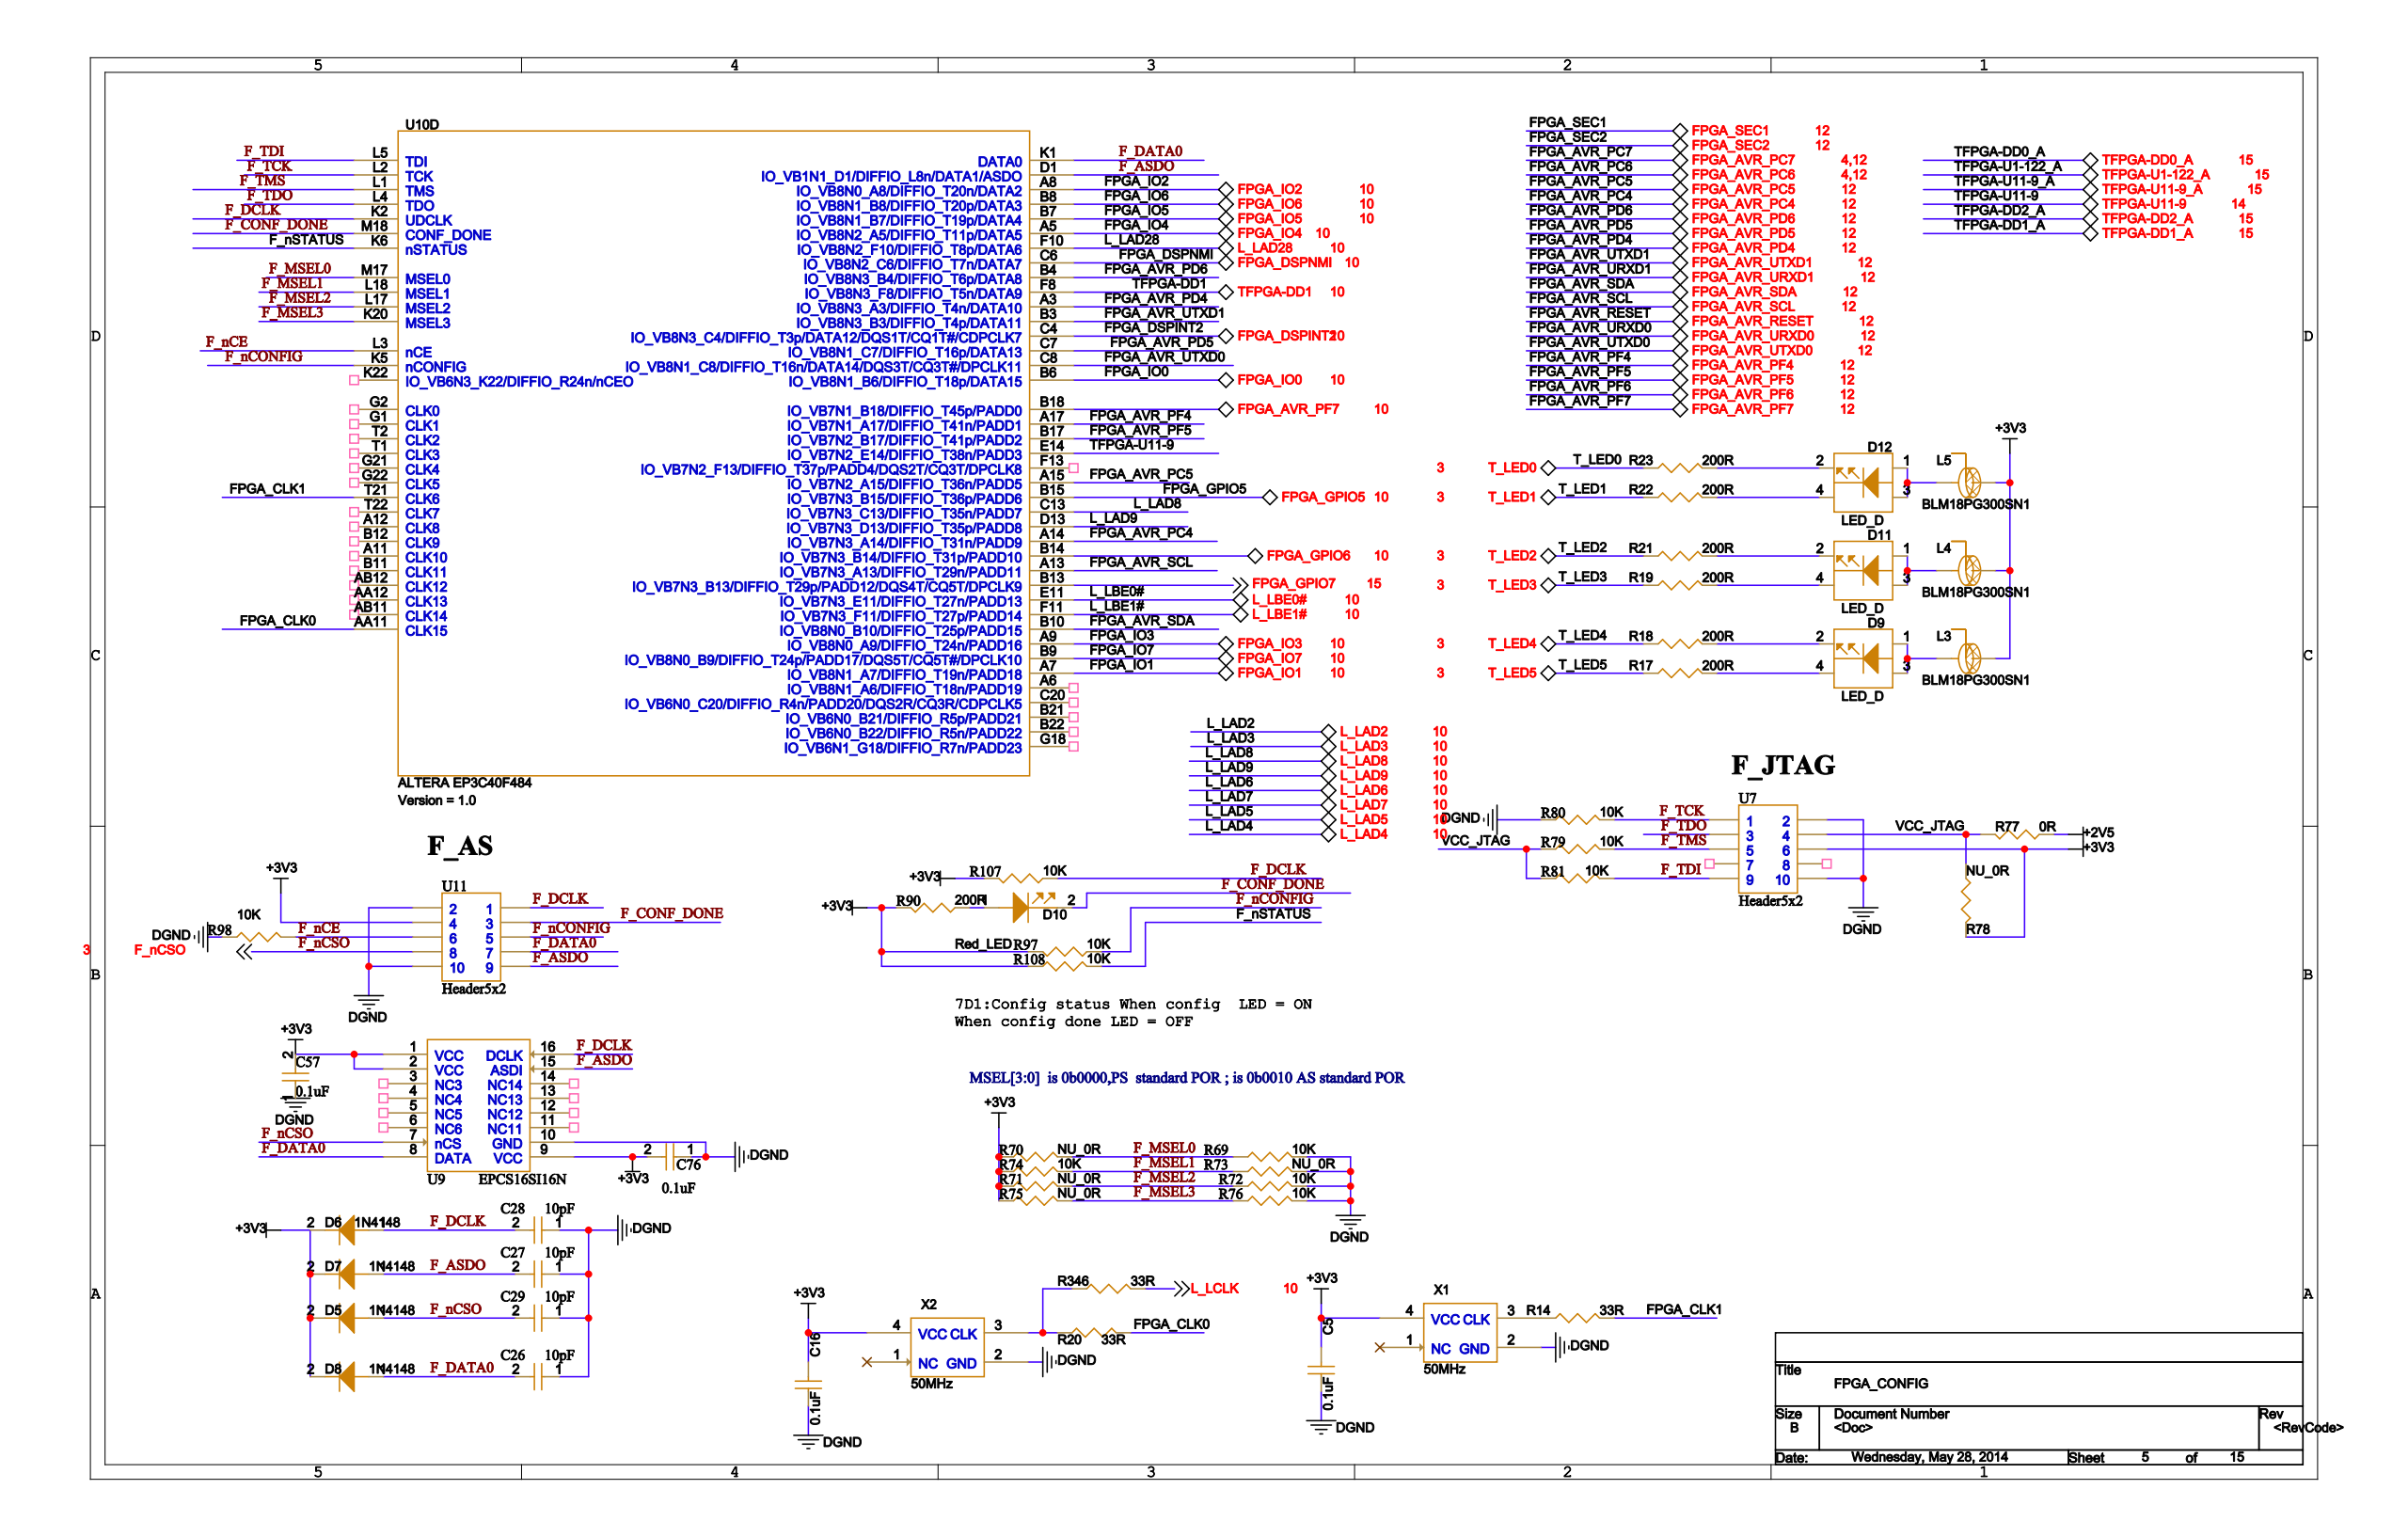Circuit board | Cadence Allegro | 669 parts | 806 nets | one sheet of the schematic
Parts on this sheet (reference | value | footprint):
C26 | 10pF | C0402
C27 | 10pF | C0402
C28 | 10pF | C0402
C29 | 10pF | C0402
C57 | 0.1uF | C0402
C76 | 0.1uF | C0402
D5 | 1N4148 | LL34
D6 | 1N4148 | LL34
D7 | 1N4148 | LL34
D8 | 1N4148 | LL34
D9 | LED_D | LED_DL
D10 | Red_LED | D0805
D11 | LED_D | LED_DL
D12 | LED_D | LED_DL
L3 | BLM18PG300SN1 | F0603
L4 | BLM18PG300SN1 | F0603
L5 | BLM18PG300SN1 | F0603
R14 | 33R | R0603
R17 | 200R | R0603
R18 | 200R | R0603
R19 | 200R | R0603
R20 | 33R | R0603
R21 | 200R | R0603
R22 | 200R | R0603
R23 | 200R | R0603
R69 | 10K | R0603
R70 | NU_0R | R0603
R71 | NU_0R | R0603
R72 | 10K | R0603
R73 | NU_0R | R0603
R74 | 10K | R0603
R75 | NU_0R | R0603
R76 | 10K | R0603
R77 | 0R | R0603
R78 | NU_0R | R0603
R79 | 10K | R0603
R80 | 10K | R0603
R81 | 10K | R0603
R90 | 200R | R0603
R97 | 10K | R0603
R98 | 10K | R0603
R107 | 10K | R0603
R108 | 10K | R0603
R346 | 33R | R0603
U7 | Header5x2 | ZIP10
U9 | EPCS16SI16N | SO16
U10 | EP3C40F484C8N | FBGA484
U11 | Header5x2 | ZIP10
X1 | 50MHz | DIP8
X2 | 50MHz | OSC-SMD7050
Nets of these parts (net: part-pin ...):
DGND: C26-1 C27-1 C28-1 C29-1 C57-1 C76-1 R69-2 R72-2 R73-2 R76-2 R80-1 R98-1 U7-2 U7-10 U9-10 U11-2 U11-10 X1-2 X2-2 U10-C5 U10-C16 U10-D8
+3V3: C57-2 C76-2 D5-2 D6-2 D7-2 D8-2 L3-1 L4-1 L5-1 R70-1 R71-1 R74-1 R75-1 R78-1 R90-2 R97-2 R107-2 R108-1 U7-6 U9-1 U9-2 U9-9 U11-4 X1-4 X2-4
F_NCSO: C29-2 D5-1 U9-7 U11-8
T_LED1: R22-1
T_LED3: R19-1
T_LED5: R17-1
T_LED0: R23-1
T_LED2: R21-1
T_LED4: R18-1
L_LAD5: U10-R18
FPGA_CLK0: R20-2 U10-AA11
FPGA_CLK1: R14-2 U10-T21
F_CONF_DONE: D10-2 U11-3 U10-M18
F_DATA0: C26-2 D8-1 U9-8 U11-7 U10-K1
F_ASDO: C27-2 D7-1 U9-15 U11-9 U10-D1
FPGA_AVR_PF4: U10-A17
FPGA_AVR_PF7: U10-B18
FPGA_AVR_PC5: U10-A15
FPGA_AVR_PF5: U10-B17
TFPGA-U11-9: U10-E14
FPGA_AVR_SCL: U10-A13
FPGA_AVR_PC4: U10-A14
FPGA_GPIO7: U10-B13
FPGA_GPIO6: U10-B14
FPGA_GPIO5: U10-B15
L_LAD8: U10-C13
L_LAD9: U10-D13
L_LBE0#: U10-E11
L_LBE1#: U10-F11
FPGA_IO2: U10-A8
FPGA_IO3: U10-A9
FPGA_AVR_SDA: U10-B10
FPGA_IO7: U10-B9
FPGA_IO1: U10-A7
FPGA_IO0: U10-B6
FPGA_IO5: U10-B7
FPGA_IO6: U10-B8
FPGA_AVR_PD5: U10-C7
FPGA_AVR_UTXD0: U10-C8
FPGA_IO4: U10-A5
FPGA_DSPNMI: U10-C6
L_LAD28: U10-F10
FPGA_AVR_PD4: U10-A3
FPGA_AVR_UTXD1: U10-B3
FPGA_AVR_PD6: U10-B4
FPGA_DSPINT2: U10-C4
TFPGA-DD1: U10-F8
F_MSEL0: R69-1 R70-2 U10-M17
F_MSEL1: R73-1 R74-2 U10-L18
F_MSEL2: R71-2 R72-1 U10-L17
F_MSEL3: R75-2 R76-1 U10-K20
F_NCE: R98-2 U11-6 U10-L3
F_NCONFIG: R97-1 U11-5 U10-K5
F_NSTATUS: R108-2 U10-K6
F_TCK: R80-2 U7-1 U10-L2
F_TDI: R81-2 U7-9 U10-L5
F_TDO: U7-3 U10-L4
F_TMS: R79-2 U7-5 U10-L1
F_DCLK: C28-2 D6-1 R107-1 U9-16 U11-1 U10-K2
+2V5: R77-1
VCC_JTAG: R77-2 R78-2 R79-1 R81-1 U7-4
N564612190: R14-1 X1-3
N58228189: R20-1 R346-1 X2-3
N56855341: D9-4 R17-2
N56855339: D9-2 R18-2
N56850813: D11-4 R19-2
N56850804: D11-2 R21-2
N56850815: D12-4 R22-2
N56850806: D12-2 R23-2
N55145610: D10-1 R90-1
L_LCLK: R346-2
N56855337: D9-1 D9-3 L3-2
N56850802: D11-1 D11-3 L4-2
N56850800: D12-1 D12-3 L5-2